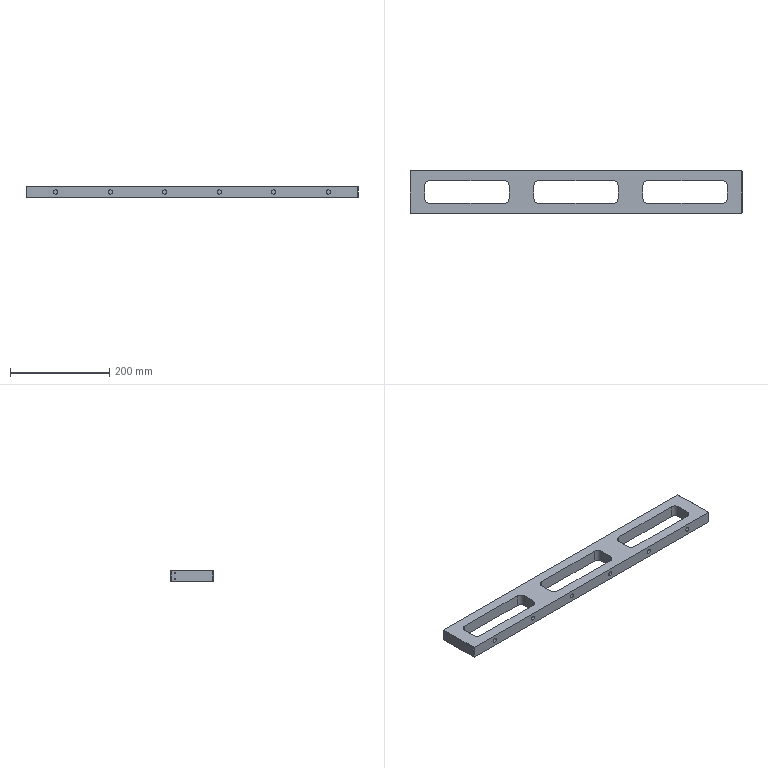Part | SolidWorks | features HoleWzd 5, Chamfer 1, Extrusion 1, ICE 1 | 1 solid | 122 faces | box 670 x 86 x 24 mm | volume 815923 mm3 | cylinder 60 | cone 36 | plane 26 | commonest cylinder face diameters 3.3 x30 9 x12 20 x12 6 x6